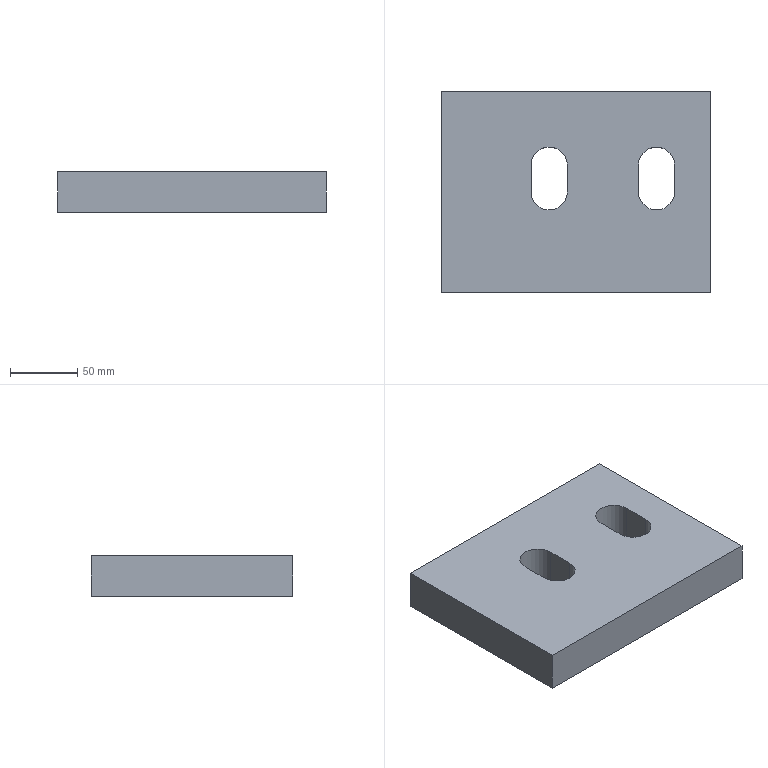Part | SolidWorks | features Extrusion 1 | 1 solid | 14 faces | box 200 x 150 x 30 mm | volume 833247 mm3 | plane 10 | cylinder 4 | commonest cylinder face diameters 27 x4
STEP:
#1=CARTESIAN_POINT('',(93.5,95.,30.));
#2=VERTEX_POINT('',#1);
#3=CARTESIAN_POINT('',(66.5,95.,30.));
#4=VERTEX_POINT('',#3);
#5=CARTESIAN_POINT('',(80.,95.,30.));
#6=DIRECTION('',(0.,0.,1.));
#7=DIRECTION('',(1.,0.,0.));
#8=AXIS2_PLACEMENT_3D('',#5,#6,#7);
#9=CIRCLE('',#8,13.5);
#10=EDGE_CURVE('',#2,#4,#9,.T.);
#11=ORIENTED_EDGE('',*,*,#10,.F.);
#12=CARTESIAN_POINT('',(93.5,75.,30.));
#13=VERTEX_POINT('',#12);
#14=CARTESIAN_POINT('',(93.5,95.,30.));
#15=DIRECTION('',(0.,1.,0.));
#16=VECTOR('',#15,1000.);
#17=LINE('',#14,#16);
#18=EDGE_CURVE('',#13,#2,#17,.T.);
#19=ORIENTED_EDGE('',*,*,#18,.F.);
#20=CARTESIAN_POINT('',(66.5,75.,30.));
#21=VERTEX_POINT('',#20);
#22=CARTESIAN_POINT('',(80.,75.,30.));
#23=DIRECTION('',(0.,0.,1.));
#24=DIRECTION('',(1.,0.,0.));
#25=AXIS2_PLACEMENT_3D('',#22,#23,#24);
#26=CIRCLE('',#25,13.5);
#27=EDGE_CURVE('',#21,#13,#26,.T.);
#28=ORIENTED_EDGE('',*,*,#27,.F.);
#29=CARTESIAN_POINT('',(66.5,95.,30.));
#30=DIRECTION('',(0.,-1.,0.));
#31=VECTOR('',#30,1000.);
#32=LINE('',#29,#31);
#33=EDGE_CURVE('',#4,#21,#32,.T.);
#34=ORIENTED_EDGE('',*,*,#33,.F.);
#35=EDGE_LOOP('',(#11,#19,#28,#34));
#36=FACE_BOUND('',#35,.T.);
#37=CARTESIAN_POINT('',(0.,150.,30.));
#38=VERTEX_POINT('',#37);
#39=CARTESIAN_POINT('',(0.,0.,30.));
#40=VERTEX_POINT('',#39);
#41=CARTESIAN_POINT('',(0.,0.,30.));
#42=DIRECTION('',(0.,-1.,0.));
#43=VECTOR('',#42,1000.);
#44=LINE('',#41,#43);
#45=EDGE_CURVE('',#38,#40,#44,.T.);
#46=ORIENTED_EDGE('',*,*,#45,.T.);
#47=CARTESIAN_POINT('',(200.,0.,30.));
#48=VERTEX_POINT('',#47);
#49=CARTESIAN_POINT('',(0.,0.,30.));
#50=DIRECTION('',(1.,0.,0.));
#51=VECTOR('',#50,1000.);
#52=LINE('',#49,#51);
#53=EDGE_CURVE('',#40,#48,#52,.T.);
#54=ORIENTED_EDGE('',*,*,#53,.T.);
#55=CARTESIAN_POINT('',(200.,150.,30.));
#56=VERTEX_POINT('',#55);
#57=CARTESIAN_POINT('',(200.,0.,30.));
#58=DIRECTION('',(0.,1.,0.));
#59=VECTOR('',#58,1000.);
#60=LINE('',#57,#59);
#61=EDGE_CURVE('',#48,#56,#60,.T.);
#62=ORIENTED_EDGE('',*,*,#61,.T.);
#63=CARTESIAN_POINT('',(0.,150.,30.));
#64=DIRECTION('',(-1.,0.,0.));
#65=VECTOR('',#64,1000.);
#66=LINE('',#63,#65);
#67=EDGE_CURVE('',#56,#38,#66,.T.);
#68=ORIENTED_EDGE('',*,*,#67,.T.);
#69=EDGE_LOOP('',(#46,#54,#62,#68));
#70=FACE_OUTER_BOUND('',#69,.T.);
#71=CARTESIAN_POINT('',(173.5,95.,30.));
#72=VERTEX_POINT('',#71);
#73=CARTESIAN_POINT('',(146.5,95.,30.));
#74=VERTEX_POINT('',#73);
#75=CARTESIAN_POINT('',(160.,95.,30.));
#76=DIRECTION('',(0.,0.,1.));
#77=DIRECTION('',(1.,0.,0.));
#78=AXIS2_PLACEMENT_3D('',#75,#76,#77);
#79=CIRCLE('',#78,13.5);
#80=EDGE_CURVE('',#72,#74,#79,.T.);
#81=ORIENTED_EDGE('',*,*,#80,.F.);
#82=CARTESIAN_POINT('',(173.5,75.,30.));
#83=VERTEX_POINT('',#82);
#84=CARTESIAN_POINT('',(173.5,95.,30.));
#85=DIRECTION('',(0.,1.,0.));
#86=VECTOR('',#85,1000.);
#87=LINE('',#84,#86);
#88=EDGE_CURVE('',#83,#72,#87,.T.);
#89=ORIENTED_EDGE('',*,*,#88,.F.);
#90=CARTESIAN_POINT('',(146.5,75.,30.));
#91=VERTEX_POINT('',#90);
#92=CARTESIAN_POINT('',(160.,75.,30.));
#93=DIRECTION('',(0.,0.,1.));
#94=DIRECTION('',(1.,0.,0.));
#95=AXIS2_PLACEMENT_3D('',#92,#93,#94);
#96=CIRCLE('',#95,13.5);
#97=EDGE_CURVE('',#91,#83,#96,.T.);
#98=ORIENTED_EDGE('',*,*,#97,.F.);
#99=CARTESIAN_POINT('',(146.5,95.,30.));
#100=DIRECTION('',(0.,-1.,0.));
#101=VECTOR('',#100,1000.);
#102=LINE('',#99,#101);
#103=EDGE_CURVE('',#74,#91,#102,.T.);
#104=ORIENTED_EDGE('',*,*,#103,.F.);
#105=EDGE_LOOP('',(#81,#89,#98,#104));
#106=FACE_BOUND('',#105,.T.);
#107=CARTESIAN_POINT('',(0.,0.,30.));
#108=DIRECTION('',(0.,0.,-1.));
#109=DIRECTION('',(-1.,0.,0.));
#110=AXIS2_PLACEMENT_3D('',#107,#108,#109);
#111=PLANE('',#110);
#112=ADVANCED_FACE('',(#36,#70,#106),#111,.F.);
#113=CARTESIAN_POINT('',(0.,150.,0.));
#114=VERTEX_POINT('',#113);
#115=CARTESIAN_POINT('',(0.,0.,0.));
#116=VERTEX_POINT('',#115);
#117=CARTESIAN_POINT('',(0.,0.,0.));
#118=DIRECTION('',(0.,-1.,0.));
#119=VECTOR('',#118,1000.);
#120=LINE('',#117,#119);
#121=EDGE_CURVE('',#114,#116,#120,.T.);
#122=ORIENTED_EDGE('',*,*,#121,.F.);
#123=CARTESIAN_POINT('',(200.,150.,0.));
#124=VERTEX_POINT('',#123);
#125=CARTESIAN_POINT('',(0.,150.,0.));
#126=DIRECTION('',(-1.,0.,0.));
#127=VECTOR('',#126,1000.);
#128=LINE('',#125,#127);
#129=EDGE_CURVE('',#124,#114,#128,.T.);
#130=ORIENTED_EDGE('',*,*,#129,.F.);
#131=CARTESIAN_POINT('',(200.,0.,0.));
#132=VERTEX_POINT('',#131);
#133=CARTESIAN_POINT('',(200.,0.,0.));
#134=DIRECTION('',(0.,1.,0.));
#135=VECTOR('',#134,1000.);
#136=LINE('',#133,#135);
#137=EDGE_CURVE('',#132,#124,#136,.T.);
#138=ORIENTED_EDGE('',*,*,#137,.F.);
#139=CARTESIAN_POINT('',(0.,0.,0.));
#140=DIRECTION('',(1.,0.,0.));
#141=VECTOR('',#140,1000.);
#142=LINE('',#139,#141);
#143=EDGE_CURVE('',#116,#132,#142,.T.);
#144=ORIENTED_EDGE('',*,*,#143,.F.);
#145=EDGE_LOOP('',(#122,#130,#138,#144));
#146=FACE_OUTER_BOUND('',#145,.T.);
#147=CARTESIAN_POINT('',(93.5,75.,0.));
#148=VERTEX_POINT('',#147);
#149=CARTESIAN_POINT('',(93.5,95.,0.));
#150=VERTEX_POINT('',#149);
#151=CARTESIAN_POINT('',(93.5,95.,0.));
#152=DIRECTION('',(0.,1.,0.));
#153=VECTOR('',#152,1000.);
#154=LINE('',#151,#153);
#155=EDGE_CURVE('',#148,#150,#154,.T.);
#156=ORIENTED_EDGE('',*,*,#155,.T.);
#157=CARTESIAN_POINT('',(66.5,95.,0.));
#158=VERTEX_POINT('',#157);
#159=CARTESIAN_POINT('',(80.,95.,0.));
#160=DIRECTION('',(0.,0.,1.));
#161=DIRECTION('',(1.,0.,0.));
#162=AXIS2_PLACEMENT_3D('',#159,#160,#161);
#163=CIRCLE('',#162,13.5);
#164=EDGE_CURVE('',#150,#158,#163,.T.);
#165=ORIENTED_EDGE('',*,*,#164,.T.);
#166=CARTESIAN_POINT('',(66.5,75.,0.));
#167=VERTEX_POINT('',#166);
#168=CARTESIAN_POINT('',(66.5,95.,0.));
#169=DIRECTION('',(0.,-1.,0.));
#170=VECTOR('',#169,1000.);
#171=LINE('',#168,#170);
#172=EDGE_CURVE('',#158,#167,#171,.T.);
#173=ORIENTED_EDGE('',*,*,#172,.T.);
#174=CARTESIAN_POINT('',(80.,75.,0.));
#175=DIRECTION('',(0.,0.,1.));
#176=DIRECTION('',(1.,0.,0.));
#177=AXIS2_PLACEMENT_3D('',#174,#175,#176);
#178=CIRCLE('',#177,13.5);
#179=EDGE_CURVE('',#167,#148,#178,.T.);
#180=ORIENTED_EDGE('',*,*,#179,.T.);
#181=EDGE_LOOP('',(#156,#165,#173,#180));
#182=FACE_BOUND('',#181,.T.);
#183=CARTESIAN_POINT('',(173.5,75.,0.));
#184=VERTEX_POINT('',#183);
#185=CARTESIAN_POINT('',(173.5,95.,0.));
#186=VERTEX_POINT('',#185);
#187=CARTESIAN_POINT('',(173.5,95.,0.));
#188=DIRECTION('',(0.,1.,0.));
#189=VECTOR('',#188,1000.);
#190=LINE('',#187,#189);
#191=EDGE_CURVE('',#184,#186,#190,.T.);
#192=ORIENTED_EDGE('',*,*,#191,.T.);
#193=CARTESIAN_POINT('',(146.5,95.,0.));
#194=VERTEX_POINT('',#193);
#195=CARTESIAN_POINT('',(160.,95.,0.));
#196=DIRECTION('',(0.,0.,1.));
#197=DIRECTION('',(1.,0.,0.));
#198=AXIS2_PLACEMENT_3D('',#195,#196,#197);
#199=CIRCLE('',#198,13.5);
#200=EDGE_CURVE('',#186,#194,#199,.T.);
#201=ORIENTED_EDGE('',*,*,#200,.T.);
#202=CARTESIAN_POINT('',(146.5,75.,0.));
#203=VERTEX_POINT('',#202);
#204=CARTESIAN_POINT('',(146.5,95.,0.));
#205=DIRECTION('',(0.,-1.,0.));
#206=VECTOR('',#205,1000.);
#207=LINE('',#204,#206);
#208=EDGE_CURVE('',#194,#203,#207,.T.);
#209=ORIENTED_EDGE('',*,*,#208,.T.);
#210=CARTESIAN_POINT('',(160.,75.,0.));
#211=DIRECTION('',(0.,0.,1.));
#212=DIRECTION('',(1.,0.,0.));
#213=AXIS2_PLACEMENT_3D('',#210,#211,#212);
#214=CIRCLE('',#213,13.5);
#215=EDGE_CURVE('',#203,#184,#214,.T.);
#216=ORIENTED_EDGE('',*,*,#215,.T.);
#217=EDGE_LOOP('',(#192,#201,#209,#216));
#218=FACE_BOUND('',#217,.T.);
#219=CARTESIAN_POINT('',(0.,0.,0.));
#220=DIRECTION('',(0.,0.,-1.));
#221=DIRECTION('',(-1.,0.,0.));
#222=AXIS2_PLACEMENT_3D('',#219,#220,#221);
#223=PLANE('',#222);
#224=ADVANCED_FACE('',(#146,#182,#218),#223,.T.);
#225=ORIENTED_EDGE('',*,*,#121,.T.);
#226=CARTESIAN_POINT('',(0.,0.,30.));
#227=DIRECTION('',(0.,0.,-1.));
#228=VECTOR('',#227,1000.);
#229=LINE('',#226,#228);
#230=EDGE_CURVE('',#40,#116,#229,.T.);
#231=ORIENTED_EDGE('',*,*,#230,.F.);
#232=ORIENTED_EDGE('',*,*,#45,.F.);
#233=CARTESIAN_POINT('',(0.,150.,30.));
#234=DIRECTION('',(0.,0.,-1.));
#235=VECTOR('',#234,1000.);
#236=LINE('',#233,#235);
#237=EDGE_CURVE('',#38,#114,#236,.T.);
#238=ORIENTED_EDGE('',*,*,#237,.T.);
#239=EDGE_LOOP('',(#225,#231,#232,#238));
#240=FACE_OUTER_BOUND('',#239,.T.);
#241=CARTESIAN_POINT('',(0.,0.,30.));
#242=DIRECTION('',(1.,0.,0.));
#243=DIRECTION('',(0.,0.,-1.));
#244=AXIS2_PLACEMENT_3D('',#241,#242,#243);
#245=PLANE('',#244);
#246=ADVANCED_FACE('',(#240),#245,.F.);
#247=ORIENTED_EDGE('',*,*,#143,.T.);
#248=CARTESIAN_POINT('',(200.,0.,30.));
#249=DIRECTION('',(0.,0.,-1.));
#250=VECTOR('',#249,1000.);
#251=LINE('',#248,#250);
#252=EDGE_CURVE('',#48,#132,#251,.T.);
#253=ORIENTED_EDGE('',*,*,#252,.F.);
#254=ORIENTED_EDGE('',*,*,#53,.F.);
#255=ORIENTED_EDGE('',*,*,#230,.T.);
#256=EDGE_LOOP('',(#247,#253,#254,#255));
#257=FACE_OUTER_BOUND('',#256,.T.);
#258=CARTESIAN_POINT('',(0.,0.,30.));
#259=DIRECTION('',(0.,1.,0.));
#260=DIRECTION('',(0.,0.,1.));
#261=AXIS2_PLACEMENT_3D('',#258,#259,#260);
#262=PLANE('',#261);
#263=ADVANCED_FACE('',(#257),#262,.F.);
#264=ORIENTED_EDGE('',*,*,#137,.T.);
#265=CARTESIAN_POINT('',(200.,150.,30.));
#266=DIRECTION('',(0.,0.,-1.));
#267=VECTOR('',#266,1000.);
#268=LINE('',#265,#267);
#269=EDGE_CURVE('',#56,#124,#268,.T.);
#270=ORIENTED_EDGE('',*,*,#269,.F.);
#271=ORIENTED_EDGE('',*,*,#61,.F.);
#272=ORIENTED_EDGE('',*,*,#252,.T.);
#273=EDGE_LOOP('',(#264,#270,#271,#272));
#274=FACE_OUTER_BOUND('',#273,.T.);
#275=CARTESIAN_POINT('',(200.,0.,30.));
#276=DIRECTION('',(-1.,0.,0.));
#277=DIRECTION('',(0.,0.,1.));
#278=AXIS2_PLACEMENT_3D('',#275,#276,#277);
#279=PLANE('',#278);
#280=ADVANCED_FACE('',(#274),#279,.F.);
#281=ORIENTED_EDGE('',*,*,#129,.T.);
#282=ORIENTED_EDGE('',*,*,#237,.F.);
#283=ORIENTED_EDGE('',*,*,#67,.F.);
#284=ORIENTED_EDGE('',*,*,#269,.T.);
#285=EDGE_LOOP('',(#281,#282,#283,#284));
#286=FACE_OUTER_BOUND('',#285,.T.);
#287=CARTESIAN_POINT('',(0.,150.,30.));
#288=DIRECTION('',(0.,-1.,0.));
#289=DIRECTION('',(0.,0.,-1.));
#290=AXIS2_PLACEMENT_3D('',#287,#288,#289);
#291=PLANE('',#290);
#292=ADVANCED_FACE('',(#286),#291,.F.);
#293=ORIENTED_EDGE('',*,*,#164,.F.);
#294=CARTESIAN_POINT('',(93.5,95.,30.));
#295=DIRECTION('',(0.,0.,-1.));
#296=VECTOR('',#295,1000.);
#297=LINE('',#294,#296);
#298=EDGE_CURVE('',#2,#150,#297,.T.);
#299=ORIENTED_EDGE('',*,*,#298,.F.);
#300=ORIENTED_EDGE('',*,*,#10,.T.);
#301=CARTESIAN_POINT('',(66.5,95.,30.));
#302=DIRECTION('',(0.,0.,-1.));
#303=VECTOR('',#302,1000.);
#304=LINE('',#301,#303);
#305=EDGE_CURVE('',#4,#158,#304,.T.);
#306=ORIENTED_EDGE('',*,*,#305,.T.);
#307=EDGE_LOOP('',(#293,#299,#300,#306));
#308=FACE_OUTER_BOUND('',#307,.T.);
#309=CARTESIAN_POINT('',(80.,95.,30.));
#310=DIRECTION('',(0.,0.,-1.));
#311=DIRECTION('',(-1.,0.,0.));
#312=AXIS2_PLACEMENT_3D('',#309,#310,#311);
#313=CYLINDRICAL_SURFACE('',#312,13.5);
#314=ADVANCED_FACE('',(#308),#313,.F.);
#315=ORIENTED_EDGE('',*,*,#172,.F.);
#316=ORIENTED_EDGE('',*,*,#305,.F.);
#317=ORIENTED_EDGE('',*,*,#33,.T.);
#318=CARTESIAN_POINT('',(66.5,75.,30.));
#319=DIRECTION('',(0.,0.,-1.));
#320=VECTOR('',#319,1000.);
#321=LINE('',#318,#320);
#322=EDGE_CURVE('',#21,#167,#321,.T.);
#323=ORIENTED_EDGE('',*,*,#322,.T.);
#324=EDGE_LOOP('',(#315,#316,#317,#323));
#325=FACE_OUTER_BOUND('',#324,.T.);
#326=CARTESIAN_POINT('',(66.5,95.,30.));
#327=DIRECTION('',(1.,0.,0.));
#328=DIRECTION('',(0.,0.,-1.));
#329=AXIS2_PLACEMENT_3D('',#326,#327,#328);
#330=PLANE('',#329);
#331=ADVANCED_FACE('',(#325),#330,.T.);
#332=ORIENTED_EDGE('',*,*,#179,.F.);
#333=ORIENTED_EDGE('',*,*,#322,.F.);
#334=ORIENTED_EDGE('',*,*,#27,.T.);
#335=CARTESIAN_POINT('',(93.5,75.,30.));
#336=DIRECTION('',(0.,0.,-1.));
#337=VECTOR('',#336,1000.);
#338=LINE('',#335,#337);
#339=EDGE_CURVE('',#13,#148,#338,.T.);
#340=ORIENTED_EDGE('',*,*,#339,.T.);
#341=EDGE_LOOP('',(#332,#333,#334,#340));
#342=FACE_OUTER_BOUND('',#341,.T.);
#343=CARTESIAN_POINT('',(80.,75.,30.));
#344=DIRECTION('',(0.,0.,-1.));
#345=DIRECTION('',(-1.,0.,0.));
#346=AXIS2_PLACEMENT_3D('',#343,#344,#345);
#347=CYLINDRICAL_SURFACE('',#346,13.5);
#348=ADVANCED_FACE('',(#342),#347,.F.);
#349=ORIENTED_EDGE('',*,*,#155,.F.);
#350=ORIENTED_EDGE('',*,*,#339,.F.);
#351=ORIENTED_EDGE('',*,*,#18,.T.);
#352=ORIENTED_EDGE('',*,*,#298,.T.);
#353=EDGE_LOOP('',(#349,#350,#351,#352));
#354=FACE_OUTER_BOUND('',#353,.T.);
#355=CARTESIAN_POINT('',(93.5,95.,30.));
#356=DIRECTION('',(-1.,0.,0.));
#357=DIRECTION('',(0.,0.,1.));
#358=AXIS2_PLACEMENT_3D('',#355,#356,#357);
#359=PLANE('',#358);
#360=ADVANCED_FACE('',(#354),#359,.T.);
#361=ORIENTED_EDGE('',*,*,#200,.F.);
#362=CARTESIAN_POINT('',(173.5,95.,30.));
#363=DIRECTION('',(0.,0.,-1.));
#364=VECTOR('',#363,1000.);
#365=LINE('',#362,#364);
#366=EDGE_CURVE('',#72,#186,#365,.T.);
#367=ORIENTED_EDGE('',*,*,#366,.F.);
#368=ORIENTED_EDGE('',*,*,#80,.T.);
#369=CARTESIAN_POINT('',(146.5,95.,30.));
#370=DIRECTION('',(0.,0.,-1.));
#371=VECTOR('',#370,1000.);
#372=LINE('',#369,#371);
#373=EDGE_CURVE('',#74,#194,#372,.T.);
#374=ORIENTED_EDGE('',*,*,#373,.T.);
#375=EDGE_LOOP('',(#361,#367,#368,#374));
#376=FACE_OUTER_BOUND('',#375,.T.);
#377=CARTESIAN_POINT('',(160.,95.,30.));
#378=DIRECTION('',(0.,0.,-1.));
#379=DIRECTION('',(-1.,0.,0.));
#380=AXIS2_PLACEMENT_3D('',#377,#378,#379);
#381=CYLINDRICAL_SURFACE('',#380,13.5);
#382=ADVANCED_FACE('',(#376),#381,.F.);
#383=ORIENTED_EDGE('',*,*,#208,.F.);
#384=ORIENTED_EDGE('',*,*,#373,.F.);
#385=ORIENTED_EDGE('',*,*,#103,.T.);
#386=CARTESIAN_POINT('',(146.5,75.,30.));
#387=DIRECTION('',(0.,0.,-1.));
#388=VECTOR('',#387,1000.);
#389=LINE('',#386,#388);
#390=EDGE_CURVE('',#91,#203,#389,.T.);
#391=ORIENTED_EDGE('',*,*,#390,.T.);
#392=EDGE_LOOP('',(#383,#384,#385,#391));
#393=FACE_OUTER_BOUND('',#392,.T.);
#394=CARTESIAN_POINT('',(146.5,95.,30.));
#395=DIRECTION('',(1.,0.,0.));
#396=DIRECTION('',(0.,0.,-1.));
#397=AXIS2_PLACEMENT_3D('',#394,#395,#396);
#398=PLANE('',#397);
#399=ADVANCED_FACE('',(#393),#398,.T.);
#400=ORIENTED_EDGE('',*,*,#215,.F.);
#401=ORIENTED_EDGE('',*,*,#390,.F.);
#402=ORIENTED_EDGE('',*,*,#97,.T.);
#403=CARTESIAN_POINT('',(173.5,75.,30.));
#404=DIRECTION('',(0.,0.,-1.));
#405=VECTOR('',#404,1000.);
#406=LINE('',#403,#405);
#407=EDGE_CURVE('',#83,#184,#406,.T.);
#408=ORIENTED_EDGE('',*,*,#407,.T.);
#409=EDGE_LOOP('',(#400,#401,#402,#408));
#410=FACE_OUTER_BOUND('',#409,.T.);
#411=CARTESIAN_POINT('',(160.,75.,30.));
#412=DIRECTION('',(0.,0.,-1.));
#413=DIRECTION('',(-1.,0.,0.));
#414=AXIS2_PLACEMENT_3D('',#411,#412,#413);
#415=CYLINDRICAL_SURFACE('',#414,13.5);
#416=ADVANCED_FACE('',(#410),#415,.F.);
#417=ORIENTED_EDGE('',*,*,#191,.F.);
#418=ORIENTED_EDGE('',*,*,#407,.F.);
#419=ORIENTED_EDGE('',*,*,#88,.T.);
#420=ORIENTED_EDGE('',*,*,#366,.T.);
#421=EDGE_LOOP('',(#417,#418,#419,#420));
#422=FACE_OUTER_BOUND('',#421,.T.);
#423=CARTESIAN_POINT('',(173.5,95.,30.));
#424=DIRECTION('',(-1.,0.,0.));
#425=DIRECTION('',(0.,0.,1.));
#426=AXIS2_PLACEMENT_3D('',#423,#424,#425);
#427=PLANE('',#426);
#428=ADVANCED_FACE('',(#422),#427,.T.);
#429=CLOSED_SHELL('',(#112,#224,#246,#263,#280,#292,#314,#331,#348,#360,#382,#399,#416,#428));
#430=MANIFOLD_SOLID_BREP('',#429);
#431=CARTESIAN_POINT('',(0.,0.,0.));
#432=DIRECTION('',(0.,0.,1.));
#433=DIRECTION('',(1.,0.,0.));
#434=AXIS2_PLACEMENT_3D('',#431,#432,#433);
#435=(LENGTH_UNIT()NAMED_UNIT(*)SI_UNIT(.MILLI.,.METRE.));
#436=UNCERTAINTY_MEASURE_WITH_UNIT(LENGTH_MEASURE(0.00001),#435,'','');
#437=(NAMED_UNIT(*)PLANE_ANGLE_UNIT()SI_UNIT($,.RADIAN.));
#438=(NAMED_UNIT(*)SI_UNIT($,.STERADIAN.)SOLID_ANGLE_UNIT());
#439=(GEOMETRIC_REPRESENTATION_CONTEXT(3)GLOBAL_UNCERTAINTY_ASSIGNED_CONTEXT((#436))GLOBAL_UNIT_ASSIGNED_CONTEXT((#435,#437,#438))REPRESENTATION_CONTEXT('',''));
#440=ADVANCED_BREP_SHAPE_REPRESENTATION('',(#430,#434),#439);